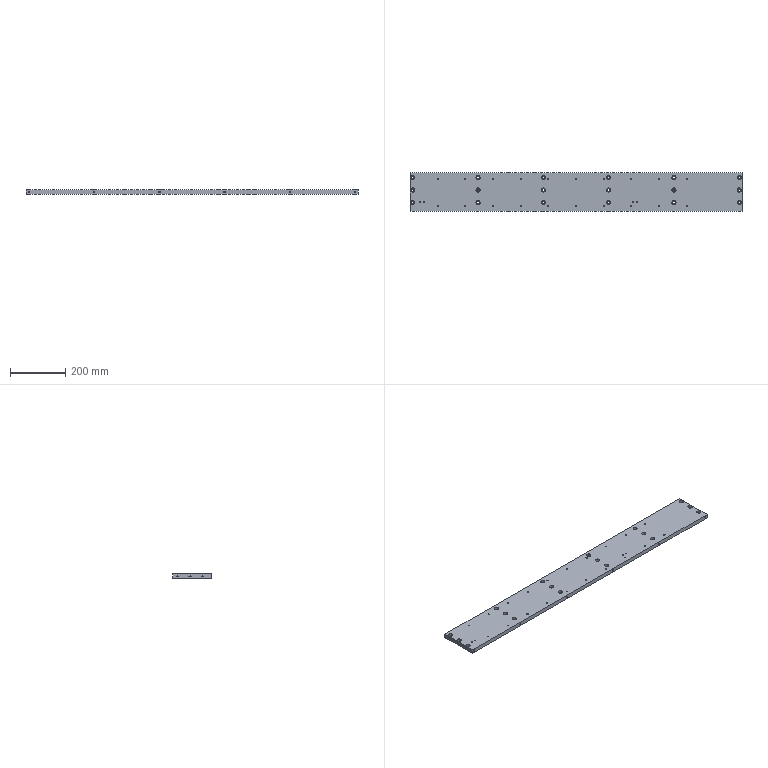Part | SolidWorks | features HoleWzd 4, LPattern 4, 3DProfileFeature 1, Extrusion 1 | 1 solid | 168 faces | box 1200 x 140 x 15 mm | volume 2477276 mm3 | cylinder 132 | plane 24 | cone 12 | commonest cylinder face diameters 4.2 x48 9 x36 15 x36 5 x12